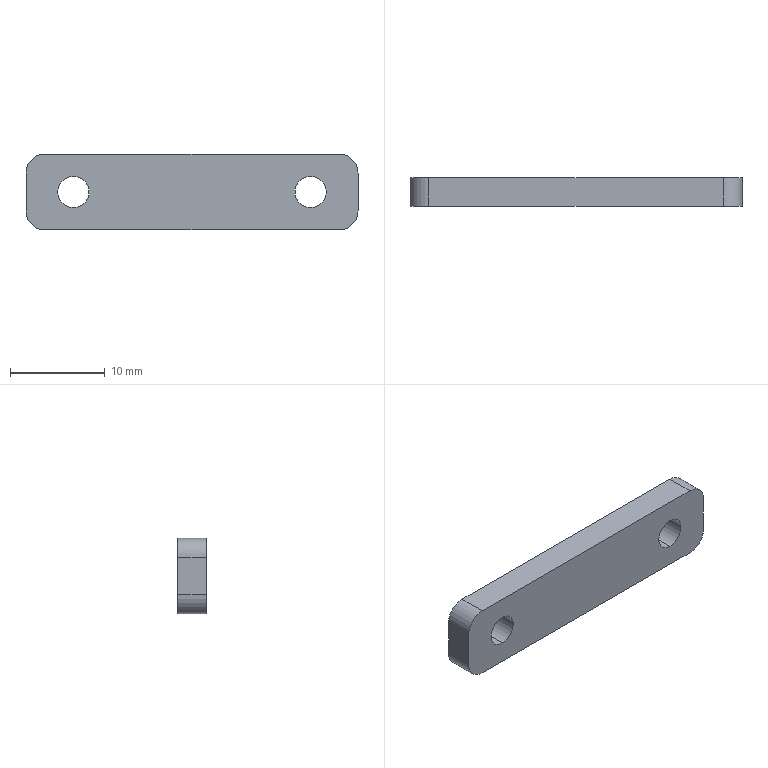Part | STEP file | 10000020560swp000-1 | 1 solid | 14 faces | box 35 x 3 x 8 mm | volume 778.381 mm3 | cylinder 8 | plane 6 | commonest cylinder face diameters 3.3 x4 4 x4
STEP:
#1=CARTESIAN_POINT('',(-12.5,0.,-1.65));
#2=VERTEX_POINT('',#1);
#3=CARTESIAN_POINT('',(-12.5,0.,1.65));
#4=VERTEX_POINT('',#3);
#5=CARTESIAN_POINT('',(-12.5,0.,0.));
#6=DIRECTION('',(0.,1.,0.));
#7=DIRECTION('',(0.,0.,1.));
#8=AXIS2_PLACEMENT_3D('',#5,#6,#7);
#9=CIRCLE('',#8,1.65);
#10=EDGE_CURVE('',#2,#4,#9,.T.);
#11=ORIENTED_EDGE('',*,*,#10,.F.);
#12=CARTESIAN_POINT('',(-12.5,3.,-1.65));
#13=VERTEX_POINT('',#12);
#14=CARTESIAN_POINT('',(-12.5,3.,-1.65));
#15=DIRECTION('',(0.,1.,0.));
#16=VECTOR('',#15,1000.);
#17=LINE('',#14,#16);
#18=EDGE_CURVE('',#2,#13,#17,.T.);
#19=ORIENTED_EDGE('',*,*,#18,.T.);
#20=CARTESIAN_POINT('',(-12.5,3.,1.65));
#21=VERTEX_POINT('',#20);
#22=CARTESIAN_POINT('',(-12.5,3.,0.));
#23=DIRECTION('',(0.,1.,0.));
#24=DIRECTION('',(0.,0.,1.));
#25=AXIS2_PLACEMENT_3D('',#22,#23,#24);
#26=CIRCLE('',#25,1.65);
#27=EDGE_CURVE('',#13,#21,#26,.T.);
#28=ORIENTED_EDGE('',*,*,#27,.T.);
#29=CARTESIAN_POINT('',(-12.5,3.,1.65));
#30=DIRECTION('',(0.,1.,0.));
#31=VECTOR('',#30,1000.);
#32=LINE('',#29,#31);
#33=EDGE_CURVE('',#4,#21,#32,.T.);
#34=ORIENTED_EDGE('',*,*,#33,.F.);
#35=EDGE_LOOP('',(#11,#19,#28,#34));
#36=FACE_OUTER_BOUND('',#35,.T.);
#37=CARTESIAN_POINT('',(-12.5,3.,0.));
#38=DIRECTION('',(0.,1.,0.));
#39=DIRECTION('',(0.,0.,1.));
#40=AXIS2_PLACEMENT_3D('',#37,#38,#39);
#41=CYLINDRICAL_SURFACE('',#40,1.65);
#42=ADVANCED_FACE('',(#36),#41,.F.);
#43=CARTESIAN_POINT('',(12.5,0.,-1.65));
#44=VERTEX_POINT('',#43);
#45=CARTESIAN_POINT('',(12.5,0.,1.65));
#46=VERTEX_POINT('',#45);
#47=CARTESIAN_POINT('',(12.5,0.,0.));
#48=DIRECTION('',(0.,1.,0.));
#49=DIRECTION('',(0.,0.,1.));
#50=AXIS2_PLACEMENT_3D('',#47,#48,#49);
#51=CIRCLE('',#50,1.65);
#52=EDGE_CURVE('',#44,#46,#51,.T.);
#53=ORIENTED_EDGE('',*,*,#52,.F.);
#54=CARTESIAN_POINT('',(12.5,3.,-1.65));
#55=VERTEX_POINT('',#54);
#56=CARTESIAN_POINT('',(12.5,3.,-1.65));
#57=DIRECTION('',(0.,1.,0.));
#58=VECTOR('',#57,1000.);
#59=LINE('',#56,#58);
#60=EDGE_CURVE('',#44,#55,#59,.T.);
#61=ORIENTED_EDGE('',*,*,#60,.T.);
#62=CARTESIAN_POINT('',(12.5,3.,1.65));
#63=VERTEX_POINT('',#62);
#64=CARTESIAN_POINT('',(12.5,3.,0.));
#65=DIRECTION('',(0.,1.,0.));
#66=DIRECTION('',(0.,0.,1.));
#67=AXIS2_PLACEMENT_3D('',#64,#65,#66);
#68=CIRCLE('',#67,1.65);
#69=EDGE_CURVE('',#55,#63,#68,.T.);
#70=ORIENTED_EDGE('',*,*,#69,.T.);
#71=CARTESIAN_POINT('',(12.5,3.,1.65));
#72=DIRECTION('',(0.,1.,0.));
#73=VECTOR('',#72,1000.);
#74=LINE('',#71,#73);
#75=EDGE_CURVE('',#46,#63,#74,.T.);
#76=ORIENTED_EDGE('',*,*,#75,.F.);
#77=EDGE_LOOP('',(#53,#61,#70,#76));
#78=FACE_OUTER_BOUND('',#77,.T.);
#79=CARTESIAN_POINT('',(12.5,3.,0.));
#80=DIRECTION('',(0.,1.,0.));
#81=DIRECTION('',(0.,0.,1.));
#82=AXIS2_PLACEMENT_3D('',#79,#80,#81);
#83=CYLINDRICAL_SURFACE('',#82,1.65);
#84=ADVANCED_FACE('',(#78),#83,.F.);
#85=CARTESIAN_POINT('',(17.5,0.,2.));
#86=VERTEX_POINT('',#85);
#87=CARTESIAN_POINT('',(17.5,0.,-2.));
#88=VERTEX_POINT('',#87);
#89=CARTESIAN_POINT('',(17.5,0.,-4.));
#90=DIRECTION('',(0.,0.,-1.));
#91=VECTOR('',#90,1000.);
#92=LINE('',#89,#91);
#93=EDGE_CURVE('',#86,#88,#92,.T.);
#94=ORIENTED_EDGE('',*,*,#93,.T.);
#95=CARTESIAN_POINT('',(17.5,3.,-2.));
#96=VERTEX_POINT('',#95);
#97=CARTESIAN_POINT('',(17.5,3.,-2.));
#98=DIRECTION('',(0.,1.,0.));
#99=VECTOR('',#98,1000.);
#100=LINE('',#97,#99);
#101=EDGE_CURVE('',#88,#96,#100,.T.);
#102=ORIENTED_EDGE('',*,*,#101,.T.);
#103=CARTESIAN_POINT('',(17.5,3.,2.));
#104=VERTEX_POINT('',#103);
#105=CARTESIAN_POINT('',(17.5,3.,-4.));
#106=DIRECTION('',(0.,0.,-1.));
#107=VECTOR('',#106,1000.);
#108=LINE('',#105,#107);
#109=EDGE_CURVE('',#104,#96,#108,.T.);
#110=ORIENTED_EDGE('',*,*,#109,.F.);
#111=CARTESIAN_POINT('',(17.5,3.,2.));
#112=DIRECTION('',(0.,-1.,0.));
#113=VECTOR('',#112,1000.);
#114=LINE('',#111,#113);
#115=EDGE_CURVE('',#104,#86,#114,.T.);
#116=ORIENTED_EDGE('',*,*,#115,.T.);
#117=EDGE_LOOP('',(#94,#102,#110,#116));
#118=FACE_OUTER_BOUND('',#117,.T.);
#119=CARTESIAN_POINT('',(17.5,3.,-4.));
#120=DIRECTION('',(-1.,0.,0.));
#121=DIRECTION('',(0.,0.,1.));
#122=AXIS2_PLACEMENT_3D('',#119,#120,#121);
#123=PLANE('',#122);
#124=ADVANCED_FACE('',(#118),#123,.F.);
#125=CARTESIAN_POINT('',(15.5,0.,-4.));
#126=VERTEX_POINT('',#125);
#127=CARTESIAN_POINT('',(-15.5,0.,-4.));
#128=VERTEX_POINT('',#127);
#129=CARTESIAN_POINT('',(-17.5,0.,-4.));
#130=DIRECTION('',(-1.,0.,0.));
#131=VECTOR('',#130,1000.);
#132=LINE('',#129,#131);
#133=EDGE_CURVE('',#126,#128,#132,.T.);
#134=ORIENTED_EDGE('',*,*,#133,.T.);
#135=CARTESIAN_POINT('',(-15.5,3.,-4.));
#136=VERTEX_POINT('',#135);
#137=CARTESIAN_POINT('',(-15.5,3.,-4.));
#138=DIRECTION('',(0.,1.,0.));
#139=VECTOR('',#138,1000.);
#140=LINE('',#137,#139);
#141=EDGE_CURVE('',#128,#136,#140,.T.);
#142=ORIENTED_EDGE('',*,*,#141,.T.);
#143=CARTESIAN_POINT('',(15.5,3.,-4.));
#144=VERTEX_POINT('',#143);
#145=CARTESIAN_POINT('',(-17.5,3.,-4.));
#146=DIRECTION('',(-1.,0.,0.));
#147=VECTOR('',#146,1000.);
#148=LINE('',#145,#147);
#149=EDGE_CURVE('',#144,#136,#148,.T.);
#150=ORIENTED_EDGE('',*,*,#149,.F.);
#151=CARTESIAN_POINT('',(15.5,3.,-4.));
#152=DIRECTION('',(0.,-1.,0.));
#153=VECTOR('',#152,1000.);
#154=LINE('',#151,#153);
#155=EDGE_CURVE('',#144,#126,#154,.T.);
#156=ORIENTED_EDGE('',*,*,#155,.T.);
#157=EDGE_LOOP('',(#134,#142,#150,#156));
#158=FACE_OUTER_BOUND('',#157,.T.);
#159=CARTESIAN_POINT('',(-17.5,3.,-4.));
#160=DIRECTION('',(0.,0.,1.));
#161=DIRECTION('',(1.,0.,0.));
#162=AXIS2_PLACEMENT_3D('',#159,#160,#161);
#163=PLANE('',#162);
#164=ADVANCED_FACE('',(#158),#163,.F.);
#165=CARTESIAN_POINT('',(-17.5,0.,-2.));
#166=VERTEX_POINT('',#165);
#167=CARTESIAN_POINT('',(-17.5,0.,2.));
#168=VERTEX_POINT('',#167);
#169=CARTESIAN_POINT('',(-17.5,0.,-4.));
#170=DIRECTION('',(0.,0.,1.));
#171=VECTOR('',#170,1000.);
#172=LINE('',#169,#171);
#173=EDGE_CURVE('',#166,#168,#172,.T.);
#174=ORIENTED_EDGE('',*,*,#173,.T.);
#175=CARTESIAN_POINT('',(-17.5,3.,2.));
#176=VERTEX_POINT('',#175);
#177=CARTESIAN_POINT('',(-17.5,3.,2.));
#178=DIRECTION('',(0.,1.,0.));
#179=VECTOR('',#178,1000.);
#180=LINE('',#177,#179);
#181=EDGE_CURVE('',#168,#176,#180,.T.);
#182=ORIENTED_EDGE('',*,*,#181,.T.);
#183=CARTESIAN_POINT('',(-17.5,3.,-2.));
#184=VERTEX_POINT('',#183);
#185=CARTESIAN_POINT('',(-17.5,3.,-4.));
#186=DIRECTION('',(0.,0.,1.));
#187=VECTOR('',#186,1000.);
#188=LINE('',#185,#187);
#189=EDGE_CURVE('',#184,#176,#188,.T.);
#190=ORIENTED_EDGE('',*,*,#189,.F.);
#191=CARTESIAN_POINT('',(-17.5,3.,-2.));
#192=DIRECTION('',(0.,-1.,0.));
#193=VECTOR('',#192,1000.);
#194=LINE('',#191,#193);
#195=EDGE_CURVE('',#184,#166,#194,.T.);
#196=ORIENTED_EDGE('',*,*,#195,.T.);
#197=EDGE_LOOP('',(#174,#182,#190,#196));
#198=FACE_OUTER_BOUND('',#197,.T.);
#199=CARTESIAN_POINT('',(-17.5,3.,-4.));
#200=DIRECTION('',(1.,0.,0.));
#201=DIRECTION('',(0.,0.,-1.));
#202=AXIS2_PLACEMENT_3D('',#199,#200,#201);
#203=PLANE('',#202);
#204=ADVANCED_FACE('',(#198),#203,.F.);
#205=CARTESIAN_POINT('',(-15.5,3.,4.));
#206=VERTEX_POINT('',#205);
#207=CARTESIAN_POINT('',(15.5,3.,4.));
#208=VERTEX_POINT('',#207);
#209=CARTESIAN_POINT('',(-17.5,3.,4.));
#210=DIRECTION('',(1.,0.,0.));
#211=VECTOR('',#210,1000.);
#212=LINE('',#209,#211);
#213=EDGE_CURVE('',#206,#208,#212,.T.);
#214=ORIENTED_EDGE('',*,*,#213,.F.);
#215=CARTESIAN_POINT('',(-15.5,0.,4.));
#216=VERTEX_POINT('',#215);
#217=CARTESIAN_POINT('',(-15.5,3.,4.));
#218=DIRECTION('',(0.,-1.,0.));
#219=VECTOR('',#218,1000.);
#220=LINE('',#217,#219);
#221=EDGE_CURVE('',#206,#216,#220,.T.);
#222=ORIENTED_EDGE('',*,*,#221,.T.);
#223=CARTESIAN_POINT('',(15.5,0.,4.));
#224=VERTEX_POINT('',#223);
#225=CARTESIAN_POINT('',(-17.5,0.,4.));
#226=DIRECTION('',(1.,0.,0.));
#227=VECTOR('',#226,1000.);
#228=LINE('',#225,#227);
#229=EDGE_CURVE('',#216,#224,#228,.T.);
#230=ORIENTED_EDGE('',*,*,#229,.T.);
#231=CARTESIAN_POINT('',(15.5,3.,4.));
#232=DIRECTION('',(0.,1.,0.));
#233=VECTOR('',#232,1000.);
#234=LINE('',#231,#233);
#235=EDGE_CURVE('',#224,#208,#234,.T.);
#236=ORIENTED_EDGE('',*,*,#235,.T.);
#237=EDGE_LOOP('',(#214,#222,#230,#236));
#238=FACE_OUTER_BOUND('',#237,.T.);
#239=CARTESIAN_POINT('',(-17.5,3.,4.));
#240=DIRECTION('',(0.,0.,-1.));
#241=DIRECTION('',(-1.,0.,0.));
#242=AXIS2_PLACEMENT_3D('',#239,#240,#241);
#243=PLANE('',#242);
#244=ADVANCED_FACE('',(#238),#243,.F.);
#245=CARTESIAN_POINT('',(-12.5,3.,0.));
#246=DIRECTION('',(0.,1.,0.));
#247=DIRECTION('',(0.,0.,1.));
#248=AXIS2_PLACEMENT_3D('',#245,#246,#247);
#249=CIRCLE('',#248,1.65);
#250=EDGE_CURVE('',#21,#13,#249,.T.);
#251=ORIENTED_EDGE('',*,*,#250,.F.);
#252=ORIENTED_EDGE('',*,*,#27,.F.);
#253=EDGE_LOOP('',(#251,#252));
#254=FACE_BOUND('',#253,.T.);
#255=CARTESIAN_POINT('',(12.5,3.,0.));
#256=DIRECTION('',(0.,1.,0.));
#257=DIRECTION('',(0.,0.,1.));
#258=AXIS2_PLACEMENT_3D('',#255,#256,#257);
#259=CIRCLE('',#258,1.65);
#260=EDGE_CURVE('',#63,#55,#259,.T.);
#261=ORIENTED_EDGE('',*,*,#260,.F.);
#262=ORIENTED_EDGE('',*,*,#69,.F.);
#263=EDGE_LOOP('',(#261,#262));
#264=FACE_BOUND('',#263,.T.);
#265=ORIENTED_EDGE('',*,*,#189,.T.);
#266=CARTESIAN_POINT('',(-15.5,3.,2.));
#267=DIRECTION('',(0.,1.,0.));
#268=DIRECTION('',(0.,0.,1.));
#269=AXIS2_PLACEMENT_3D('',#266,#267,#268);
#270=CIRCLE('',#269,2.);
#271=EDGE_CURVE('',#176,#206,#270,.T.);
#272=ORIENTED_EDGE('',*,*,#271,.T.);
#273=ORIENTED_EDGE('',*,*,#213,.T.);
#274=CARTESIAN_POINT('',(15.5,3.,2.));
#275=DIRECTION('',(0.,1.,0.));
#276=DIRECTION('',(0.,0.,1.));
#277=AXIS2_PLACEMENT_3D('',#274,#275,#276);
#278=CIRCLE('',#277,2.);
#279=EDGE_CURVE('',#208,#104,#278,.T.);
#280=ORIENTED_EDGE('',*,*,#279,.T.);
#281=ORIENTED_EDGE('',*,*,#109,.T.);
#282=CARTESIAN_POINT('',(15.5,3.,-2.));
#283=DIRECTION('',(0.,1.,0.));
#284=DIRECTION('',(0.,0.,1.));
#285=AXIS2_PLACEMENT_3D('',#282,#283,#284);
#286=CIRCLE('',#285,2.);
#287=EDGE_CURVE('',#96,#144,#286,.T.);
#288=ORIENTED_EDGE('',*,*,#287,.T.);
#289=ORIENTED_EDGE('',*,*,#149,.T.);
#290=CARTESIAN_POINT('',(-15.5,3.,-2.));
#291=DIRECTION('',(0.,1.,0.));
#292=DIRECTION('',(0.,0.,1.));
#293=AXIS2_PLACEMENT_3D('',#290,#291,#292);
#294=CIRCLE('',#293,2.);
#295=EDGE_CURVE('',#136,#184,#294,.T.);
#296=ORIENTED_EDGE('',*,*,#295,.T.);
#297=EDGE_LOOP('',(#265,#272,#273,#280,#281,#288,#289,#296));
#298=FACE_OUTER_BOUND('',#297,.T.);
#299=CARTESIAN_POINT('',(0.,3.,0.));
#300=DIRECTION('',(0.,1.,0.));
#301=DIRECTION('',(0.,0.,1.));
#302=AXIS2_PLACEMENT_3D('',#299,#300,#301);
#303=PLANE('',#302);
#304=ADVANCED_FACE('',(#254,#264,#298),#303,.T.);
#305=CARTESIAN_POINT('',(-12.5,0.,0.));
#306=DIRECTION('',(0.,1.,0.));
#307=DIRECTION('',(0.,0.,1.));
#308=AXIS2_PLACEMENT_3D('',#305,#306,#307);
#309=CIRCLE('',#308,1.65);
#310=EDGE_CURVE('',#4,#2,#309,.T.);
#311=ORIENTED_EDGE('',*,*,#310,.T.);
#312=ORIENTED_EDGE('',*,*,#10,.T.);
#313=EDGE_LOOP('',(#311,#312));
#314=FACE_BOUND('',#313,.T.);
#315=CARTESIAN_POINT('',(12.5,0.,0.));
#316=DIRECTION('',(0.,1.,0.));
#317=DIRECTION('',(0.,0.,1.));
#318=AXIS2_PLACEMENT_3D('',#315,#316,#317);
#319=CIRCLE('',#318,1.65);
#320=EDGE_CURVE('',#46,#44,#319,.T.);
#321=ORIENTED_EDGE('',*,*,#320,.T.);
#322=ORIENTED_EDGE('',*,*,#52,.T.);
#323=EDGE_LOOP('',(#321,#322));
#324=FACE_BOUND('',#323,.T.);
#325=ORIENTED_EDGE('',*,*,#229,.F.);
#326=CARTESIAN_POINT('',(-15.5,0.,2.));
#327=DIRECTION('',(0.,-1.,0.));
#328=DIRECTION('',(0.,0.,1.));
#329=AXIS2_PLACEMENT_3D('',#326,#327,#328);
#330=CIRCLE('',#329,2.);
#331=EDGE_CURVE('',#216,#168,#330,.T.);
#332=ORIENTED_EDGE('',*,*,#331,.T.);
#333=ORIENTED_EDGE('',*,*,#173,.F.);
#334=CARTESIAN_POINT('',(-15.5,0.,-2.));
#335=DIRECTION('',(0.,-1.,0.));
#336=DIRECTION('',(0.,0.,1.));
#337=AXIS2_PLACEMENT_3D('',#334,#335,#336);
#338=CIRCLE('',#337,2.);
#339=EDGE_CURVE('',#166,#128,#338,.T.);
#340=ORIENTED_EDGE('',*,*,#339,.T.);
#341=ORIENTED_EDGE('',*,*,#133,.F.);
#342=CARTESIAN_POINT('',(15.5,0.,-2.));
#343=DIRECTION('',(0.,-1.,0.));
#344=DIRECTION('',(0.,0.,1.));
#345=AXIS2_PLACEMENT_3D('',#342,#343,#344);
#346=CIRCLE('',#345,2.);
#347=EDGE_CURVE('',#126,#88,#346,.T.);
#348=ORIENTED_EDGE('',*,*,#347,.T.);
#349=ORIENTED_EDGE('',*,*,#93,.F.);
#350=CARTESIAN_POINT('',(15.5,0.,2.));
#351=DIRECTION('',(0.,-1.,0.));
#352=DIRECTION('',(0.,0.,1.));
#353=AXIS2_PLACEMENT_3D('',#350,#351,#352);
#354=CIRCLE('',#353,2.);
#355=EDGE_CURVE('',#86,#224,#354,.T.);
#356=ORIENTED_EDGE('',*,*,#355,.T.);
#357=EDGE_LOOP('',(#325,#332,#333,#340,#341,#348,#349,#356));
#358=FACE_OUTER_BOUND('',#357,.T.);
#359=CARTESIAN_POINT('',(0.,0.,0.));
#360=DIRECTION('',(0.,1.,0.));
#361=DIRECTION('',(0.,0.,1.));
#362=AXIS2_PLACEMENT_3D('',#359,#360,#361);
#363=PLANE('',#362);
#364=ADVANCED_FACE('',(#314,#324,#358),#363,.F.);
#365=ORIENTED_EDGE('',*,*,#60,.F.);
#366=ORIENTED_EDGE('',*,*,#320,.F.);
#367=ORIENTED_EDGE('',*,*,#75,.T.);
#368=ORIENTED_EDGE('',*,*,#260,.T.);
#369=EDGE_LOOP('',(#365,#366,#367,#368));
#370=FACE_OUTER_BOUND('',#369,.T.);
#371=CARTESIAN_POINT('',(12.5,3.,0.));
#372=DIRECTION('',(0.,1.,0.));
#373=DIRECTION('',(0.,0.,1.));
#374=AXIS2_PLACEMENT_3D('',#371,#372,#373);
#375=CYLINDRICAL_SURFACE('',#374,1.65);
#376=ADVANCED_FACE('',(#370),#375,.F.);
#377=ORIENTED_EDGE('',*,*,#18,.F.);
#378=ORIENTED_EDGE('',*,*,#310,.F.);
#379=ORIENTED_EDGE('',*,*,#33,.T.);
#380=ORIENTED_EDGE('',*,*,#250,.T.);
#381=EDGE_LOOP('',(#377,#378,#379,#380));
#382=FACE_OUTER_BOUND('',#381,.T.);
#383=CARTESIAN_POINT('',(-12.5,3.,0.));
#384=DIRECTION('',(0.,1.,0.));
#385=DIRECTION('',(0.,0.,1.));
#386=AXIS2_PLACEMENT_3D('',#383,#384,#385);
#387=CYLINDRICAL_SURFACE('',#386,1.65);
#388=ADVANCED_FACE('',(#382),#387,.F.);
#389=ORIENTED_EDGE('',*,*,#271,.F.);
#390=ORIENTED_EDGE('',*,*,#181,.F.);
#391=ORIENTED_EDGE('',*,*,#331,.F.);
#392=ORIENTED_EDGE('',*,*,#221,.F.);
#393=EDGE_LOOP('',(#389,#390,#391,#392));
#394=FACE_OUTER_BOUND('',#393,.T.);
#395=CARTESIAN_POINT('',(-15.5,3.,2.));
#396=DIRECTION('',(0.,-1.,0.));
#397=DIRECTION('',(0.,0.,-1.));
#398=AXIS2_PLACEMENT_3D('',#395,#396,#397);
#399=CYLINDRICAL_SURFACE('',#398,2.);
#400=ADVANCED_FACE('',(#394),#399,.T.);
#401=ORIENTED_EDGE('',*,*,#295,.F.);
#402=ORIENTED_EDGE('',*,*,#141,.F.);
#403=ORIENTED_EDGE('',*,*,#339,.F.);
#404=ORIENTED_EDGE('',*,*,#195,.F.);
#405=EDGE_LOOP('',(#401,#402,#403,#404));
#406=FACE_OUTER_BOUND('',#405,.T.);
#407=CARTESIAN_POINT('',(-15.5,3.,-2.));
#408=DIRECTION('',(0.,-1.,0.));
#409=DIRECTION('',(0.,0.,-1.));
#410=AXIS2_PLACEMENT_3D('',#407,#408,#409);
#411=CYLINDRICAL_SURFACE('',#410,2.);
#412=ADVANCED_FACE('',(#406),#411,.T.);
#413=ORIENTED_EDGE('',*,*,#287,.F.);
#414=ORIENTED_EDGE('',*,*,#101,.F.);
#415=ORIENTED_EDGE('',*,*,#347,.F.);
#416=ORIENTED_EDGE('',*,*,#155,.F.);
#417=EDGE_LOOP('',(#413,#414,#415,#416));
#418=FACE_OUTER_BOUND('',#417,.T.);
#419=CARTESIAN_POINT('',(15.5,3.,-2.));
#420=DIRECTION('',(0.,-1.,0.));
#421=DIRECTION('',(0.,0.,-1.));
#422=AXIS2_PLACEMENT_3D('',#419,#420,#421);
#423=CYLINDRICAL_SURFACE('',#422,2.);
#424=ADVANCED_FACE('',(#418),#423,.T.);
#425=ORIENTED_EDGE('',*,*,#279,.F.);
#426=ORIENTED_EDGE('',*,*,#235,.F.);
#427=ORIENTED_EDGE('',*,*,#355,.F.);
#428=ORIENTED_EDGE('',*,*,#115,.F.);
#429=EDGE_LOOP('',(#425,#426,#427,#428));
#430=FACE_OUTER_BOUND('',#429,.T.);
#431=CARTESIAN_POINT('',(15.5,3.,2.));
#432=DIRECTION('',(0.,-1.,0.));
#433=DIRECTION('',(0.,0.,-1.));
#434=AXIS2_PLACEMENT_3D('',#431,#432,#433);
#435=CYLINDRICAL_SURFACE('',#434,2.);
#436=ADVANCED_FACE('',(#430),#435,.T.);
#437=CLOSED_SHELL('',(#42,#84,#124,#164,#204,#244,#304,#364,#376,#388,#400,#412,#424,#436));
#438=MANIFOLD_SOLID_BREP('',#437);
#439=CARTESIAN_POINT('',(0.,0.,0.));
#440=DIRECTION('',(0.,0.,1.));
#441=DIRECTION('',(1.,0.,0.));
#442=AXIS2_PLACEMENT_3D('',#439,#440,#441);
#443=(LENGTH_UNIT()NAMED_UNIT(*)SI_UNIT(.MILLI.,.METRE.));
#444=UNCERTAINTY_MEASURE_WITH_UNIT(LENGTH_MEASURE(0.00001),#443,'','');
#445=(NAMED_UNIT(*)PLANE_ANGLE_UNIT()SI_UNIT($,.RADIAN.));
#446=(NAMED_UNIT(*)SI_UNIT($,.STERADIAN.)SOLID_ANGLE_UNIT());
#447=(GEOMETRIC_REPRESENTATION_CONTEXT(3)GLOBAL_UNCERTAINTY_ASSIGNED_CONTEXT((#444))GLOBAL_UNIT_ASSIGNED_CONTEXT((#443,#445,#446))REPRESENTATION_CONTEXT('',''));
#448=ADVANCED_BREP_SHAPE_REPRESENTATION('',(#438,#442),#447);